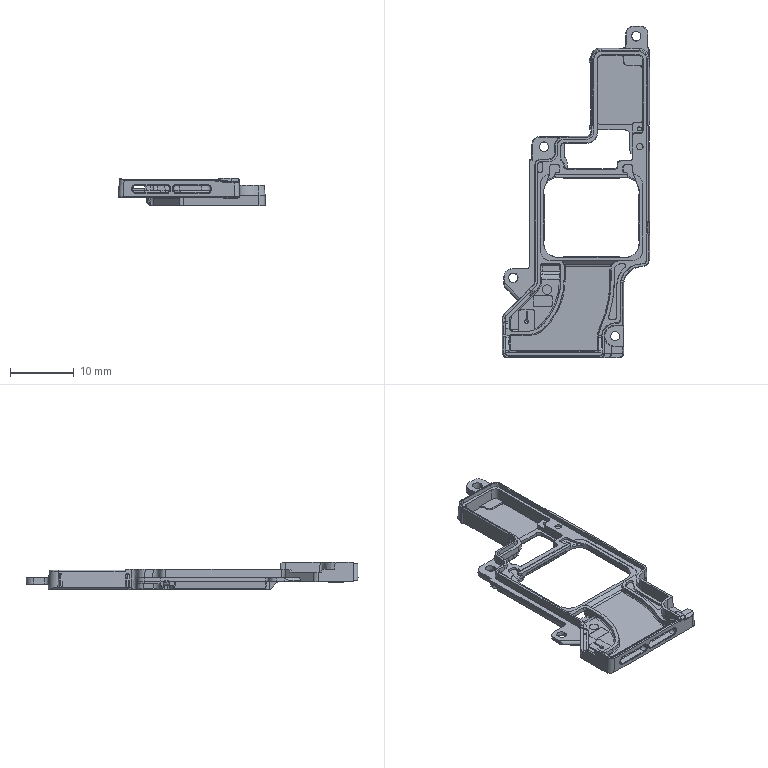Part | STEP file | N56_BOTTOM_5 | 1 solid | 881 faces | box 23.138 x 52.172 x 4.381 mm | volume 531.504 mm3 | plane 434 | cylinder 225 | cone 132 | spline 90 | commonest cylinder face diameters 0.4 x51 1 x33 0.1 x26 0.6 x20 0.3 x14 2 x12